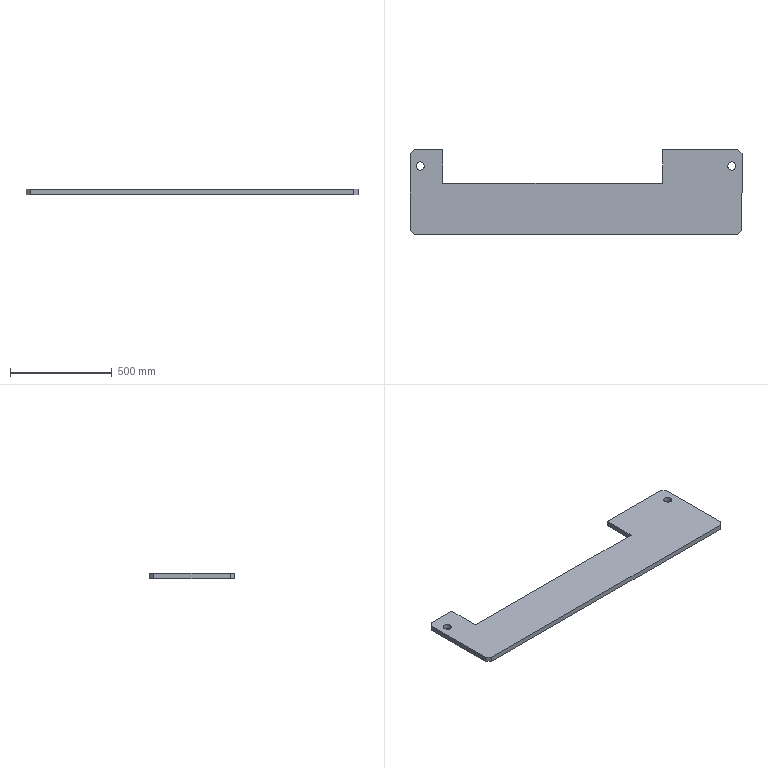Part | SolidWorks | features Chamfer 1, Extrusion 1, ICE 1 | 1 solid | 18 faces | box 1630 x 415 x 25 mm | volume 12373418 mm3 | plane 14 | cylinder 4 | commonest cylinder face diameters 40 x4
STEP:
#1=CARTESIAN_POINT('',(745.,127.5,0.));
#2=VERTEX_POINT('',#1);
#3=CARTESIAN_POINT('',(785.,127.5,0.));
#4=VERTEX_POINT('',#3);
#5=CARTESIAN_POINT('',(765.,127.5,0.));
#6=DIRECTION('',(0.,0.,1.));
#7=DIRECTION('',(1.,0.,0.));
#8=AXIS2_PLACEMENT_3D('',#5,#6,#7);
#9=CIRCLE('',#8,20.);
#10=EDGE_CURVE('',#2,#4,#9,.T.);
#11=ORIENTED_EDGE('',*,*,#10,.F.);
#12=CARTESIAN_POINT('',(745.,127.5,25.));
#13=VERTEX_POINT('',#12);
#14=CARTESIAN_POINT('',(745.,127.5,0.));
#15=DIRECTION('',(0.,0.,1.));
#16=VECTOR('',#15,1000.);
#17=LINE('',#14,#16);
#18=EDGE_CURVE('',#2,#13,#17,.T.);
#19=ORIENTED_EDGE('',*,*,#18,.T.);
#20=CARTESIAN_POINT('',(785.,127.5,25.));
#21=VERTEX_POINT('',#20);
#22=CARTESIAN_POINT('',(765.,127.5,25.));
#23=DIRECTION('',(0.,0.,-1.));
#24=DIRECTION('',(-1.,0.,0.));
#25=AXIS2_PLACEMENT_3D('',#22,#23,#24);
#26=CIRCLE('',#25,20.);
#27=EDGE_CURVE('',#21,#13,#26,.T.);
#28=ORIENTED_EDGE('',*,*,#27,.F.);
#29=CARTESIAN_POINT('',(785.,127.5,0.));
#30=DIRECTION('',(0.,0.,1.));
#31=VECTOR('',#30,1000.);
#32=LINE('',#29,#31);
#33=EDGE_CURVE('',#4,#21,#32,.T.);
#34=ORIENTED_EDGE('',*,*,#33,.F.);
#35=EDGE_LOOP('',(#11,#19,#28,#34));
#36=FACE_OUTER_BOUND('',#35,.T.);
#37=CARTESIAN_POINT('',(765.,127.5,0.));
#38=DIRECTION('',(0.,0.,1.));
#39=DIRECTION('',(1.,0.,0.));
#40=AXIS2_PLACEMENT_3D('',#37,#38,#39);
#41=CYLINDRICAL_SURFACE('',#40,20.);
#42=ADVANCED_FACE('',(#36),#41,.F.);
#43=CARTESIAN_POINT('',(-785.,127.5,0.));
#44=VERTEX_POINT('',#43);
#45=CARTESIAN_POINT('',(-745.,127.5,0.));
#46=VERTEX_POINT('',#45);
#47=CARTESIAN_POINT('',(-765.,127.5,0.));
#48=DIRECTION('',(0.,0.,1.));
#49=DIRECTION('',(1.,0.,0.));
#50=AXIS2_PLACEMENT_3D('',#47,#48,#49);
#51=CIRCLE('',#50,20.);
#52=EDGE_CURVE('',#44,#46,#51,.T.);
#53=ORIENTED_EDGE('',*,*,#52,.F.);
#54=CARTESIAN_POINT('',(-785.,127.5,25.));
#55=VERTEX_POINT('',#54);
#56=CARTESIAN_POINT('',(-785.,127.5,0.));
#57=DIRECTION('',(0.,0.,1.));
#58=VECTOR('',#57,1000.);
#59=LINE('',#56,#58);
#60=EDGE_CURVE('',#44,#55,#59,.T.);
#61=ORIENTED_EDGE('',*,*,#60,.T.);
#62=CARTESIAN_POINT('',(-745.,127.5,25.));
#63=VERTEX_POINT('',#62);
#64=CARTESIAN_POINT('',(-765.,127.5,25.));
#65=DIRECTION('',(0.,0.,-1.));
#66=DIRECTION('',(-1.,0.,0.));
#67=AXIS2_PLACEMENT_3D('',#64,#65,#66);
#68=CIRCLE('',#67,20.);
#69=EDGE_CURVE('',#63,#55,#68,.T.);
#70=ORIENTED_EDGE('',*,*,#69,.F.);
#71=CARTESIAN_POINT('',(-745.,127.5,0.));
#72=DIRECTION('',(0.,0.,1.));
#73=VECTOR('',#72,1000.);
#74=LINE('',#71,#73);
#75=EDGE_CURVE('',#46,#63,#74,.T.);
#76=ORIENTED_EDGE('',*,*,#75,.F.);
#77=EDGE_LOOP('',(#53,#61,#70,#76));
#78=FACE_OUTER_BOUND('',#77,.T.);
#79=CARTESIAN_POINT('',(-765.,127.5,0.));
#80=DIRECTION('',(0.,0.,1.));
#81=DIRECTION('',(1.,0.,0.));
#82=AXIS2_PLACEMENT_3D('',#79,#80,#81);
#83=CYLINDRICAL_SURFACE('',#82,20.);
#84=ADVANCED_FACE('',(#78),#83,.F.);
#85=CARTESIAN_POINT('',(-655.,207.5,25.));
#86=VERTEX_POINT('',#85);
#87=CARTESIAN_POINT('',(-795.,207.5,25.));
#88=VERTEX_POINT('',#87);
#89=CARTESIAN_POINT('',(815.,207.5,25.));
#90=DIRECTION('',(-1.,0.,0.));
#91=VECTOR('',#90,1000.);
#92=LINE('',#89,#91);
#93=EDGE_CURVE('',#86,#88,#92,.T.);
#94=ORIENTED_EDGE('',*,*,#93,.F.);
#95=CARTESIAN_POINT('',(-655.,207.5,0.));
#96=VERTEX_POINT('',#95);
#97=CARTESIAN_POINT('',(-655.,207.5,25.));
#98=DIRECTION('',(0.,0.,-1.));
#99=VECTOR('',#98,1000.);
#100=LINE('',#97,#99);
#101=EDGE_CURVE('',#86,#96,#100,.T.);
#102=ORIENTED_EDGE('',*,*,#101,.T.);
#103=CARTESIAN_POINT('',(-795.,207.5,0.));
#104=VERTEX_POINT('',#103);
#105=CARTESIAN_POINT('',(815.,207.5,0.));
#106=DIRECTION('',(-1.,0.,0.));
#107=VECTOR('',#106,1000.);
#108=LINE('',#105,#107);
#109=EDGE_CURVE('',#96,#104,#108,.T.);
#110=ORIENTED_EDGE('',*,*,#109,.T.);
#111=CARTESIAN_POINT('',(-795.,207.5,25.));
#112=DIRECTION('',(0.,0.,1.));
#113=VECTOR('',#112,1000.);
#114=LINE('',#111,#113);
#115=EDGE_CURVE('',#104,#88,#114,.T.);
#116=ORIENTED_EDGE('',*,*,#115,.T.);
#117=EDGE_LOOP('',(#94,#102,#110,#116));
#118=FACE_OUTER_BOUND('',#117,.T.);
#119=CARTESIAN_POINT('',(815.,207.5,25.));
#120=DIRECTION('',(0.,-1.,0.));
#121=DIRECTION('',(1.,0.,0.));
#122=AXIS2_PLACEMENT_3D('',#119,#120,#121);
#123=PLANE('',#122);
#124=ADVANCED_FACE('',(#118),#123,.F.);
#125=CARTESIAN_POINT('',(-815.,187.5,0.));
#126=VERTEX_POINT('',#125);
#127=CARTESIAN_POINT('',(-815.,-187.5,0.));
#128=VERTEX_POINT('',#127);
#129=CARTESIAN_POINT('',(-815.,207.5,0.));
#130=DIRECTION('',(0.,-1.,0.));
#131=VECTOR('',#130,1000.);
#132=LINE('',#129,#131);
#133=EDGE_CURVE('',#126,#128,#132,.T.);
#134=ORIENTED_EDGE('',*,*,#133,.T.);
#135=CARTESIAN_POINT('',(-815.,-187.5,25.));
#136=VERTEX_POINT('',#135);
#137=CARTESIAN_POINT('',(-815.,-187.5,25.));
#138=DIRECTION('',(0.,0.,1.));
#139=VECTOR('',#138,1000.);
#140=LINE('',#137,#139);
#141=EDGE_CURVE('',#128,#136,#140,.T.);
#142=ORIENTED_EDGE('',*,*,#141,.T.);
#143=CARTESIAN_POINT('',(-815.,187.5,25.));
#144=VERTEX_POINT('',#143);
#145=CARTESIAN_POINT('',(-815.,207.5,25.));
#146=DIRECTION('',(0.,-1.,0.));
#147=VECTOR('',#146,1000.);
#148=LINE('',#145,#147);
#149=EDGE_CURVE('',#144,#136,#148,.T.);
#150=ORIENTED_EDGE('',*,*,#149,.F.);
#151=CARTESIAN_POINT('',(-815.,187.5,25.));
#152=DIRECTION('',(0.,0.,-1.));
#153=VECTOR('',#152,1000.);
#154=LINE('',#151,#153);
#155=EDGE_CURVE('',#144,#126,#154,.T.);
#156=ORIENTED_EDGE('',*,*,#155,.T.);
#157=EDGE_LOOP('',(#134,#142,#150,#156));
#158=FACE_OUTER_BOUND('',#157,.T.);
#159=CARTESIAN_POINT('',(-815.,207.5,25.));
#160=DIRECTION('',(1.,0.,0.));
#161=DIRECTION('',(0.,1.,0.));
#162=AXIS2_PLACEMENT_3D('',#159,#160,#161);
#163=PLANE('',#162);
#164=ADVANCED_FACE('',(#158),#163,.F.);
#165=CARTESIAN_POINT('',(-795.,-207.5,25.));
#166=VERTEX_POINT('',#165);
#167=CARTESIAN_POINT('',(795.,-207.5,25.));
#168=VERTEX_POINT('',#167);
#169=CARTESIAN_POINT('',(815.,-207.5,25.));
#170=DIRECTION('',(1.,0.,0.));
#171=VECTOR('',#170,1000.);
#172=LINE('',#169,#171);
#173=EDGE_CURVE('',#166,#168,#172,.T.);
#174=ORIENTED_EDGE('',*,*,#173,.F.);
#175=CARTESIAN_POINT('',(-795.,-207.5,0.));
#176=VERTEX_POINT('',#175);
#177=CARTESIAN_POINT('',(-795.,-207.5,25.));
#178=DIRECTION('',(0.,0.,-1.));
#179=VECTOR('',#178,1000.);
#180=LINE('',#177,#179);
#181=EDGE_CURVE('',#166,#176,#180,.T.);
#182=ORIENTED_EDGE('',*,*,#181,.T.);
#183=CARTESIAN_POINT('',(795.,-207.5,0.));
#184=VERTEX_POINT('',#183);
#185=CARTESIAN_POINT('',(815.,-207.5,0.));
#186=DIRECTION('',(1.,0.,0.));
#187=VECTOR('',#186,1000.);
#188=LINE('',#185,#187);
#189=EDGE_CURVE('',#176,#184,#188,.T.);
#190=ORIENTED_EDGE('',*,*,#189,.T.);
#191=CARTESIAN_POINT('',(795.,-207.5,25.));
#192=DIRECTION('',(0.,0.,1.));
#193=VECTOR('',#192,1000.);
#194=LINE('',#191,#193);
#195=EDGE_CURVE('',#184,#168,#194,.T.);
#196=ORIENTED_EDGE('',*,*,#195,.T.);
#197=EDGE_LOOP('',(#174,#182,#190,#196));
#198=FACE_OUTER_BOUND('',#197,.T.);
#199=CARTESIAN_POINT('',(815.,-207.5,25.));
#200=DIRECTION('',(0.,1.,0.));
#201=DIRECTION('',(-1.,0.,0.));
#202=AXIS2_PLACEMENT_3D('',#199,#200,#201);
#203=PLANE('',#202);
#204=ADVANCED_FACE('',(#198),#203,.F.);
#205=CARTESIAN_POINT('',(815.,-187.5,25.));
#206=VERTEX_POINT('',#205);
#207=CARTESIAN_POINT('',(815.,187.5,25.));
#208=VERTEX_POINT('',#207);
#209=CARTESIAN_POINT('',(815.,207.5,25.));
#210=DIRECTION('',(0.,1.,0.));
#211=VECTOR('',#210,1000.);
#212=LINE('',#209,#211);
#213=EDGE_CURVE('',#206,#208,#212,.T.);
#214=ORIENTED_EDGE('',*,*,#213,.F.);
#215=CARTESIAN_POINT('',(815.,-187.5,0.));
#216=VERTEX_POINT('',#215);
#217=CARTESIAN_POINT('',(815.,-187.5,25.));
#218=DIRECTION('',(0.,0.,-1.));
#219=VECTOR('',#218,1000.);
#220=LINE('',#217,#219);
#221=EDGE_CURVE('',#206,#216,#220,.T.);
#222=ORIENTED_EDGE('',*,*,#221,.T.);
#223=CARTESIAN_POINT('',(815.,187.5,0.));
#224=VERTEX_POINT('',#223);
#225=CARTESIAN_POINT('',(815.,207.5,0.));
#226=DIRECTION('',(0.,1.,0.));
#227=VECTOR('',#226,1000.);
#228=LINE('',#225,#227);
#229=EDGE_CURVE('',#216,#224,#228,.T.);
#230=ORIENTED_EDGE('',*,*,#229,.T.);
#231=CARTESIAN_POINT('',(815.,187.5,25.));
#232=DIRECTION('',(0.,0.,1.));
#233=VECTOR('',#232,1000.);
#234=LINE('',#231,#233);
#235=EDGE_CURVE('',#224,#208,#234,.T.);
#236=ORIENTED_EDGE('',*,*,#235,.T.);
#237=EDGE_LOOP('',(#214,#222,#230,#236));
#238=FACE_OUTER_BOUND('',#237,.T.);
#239=CARTESIAN_POINT('',(815.,207.5,25.));
#240=DIRECTION('',(-1.,0.,0.));
#241=DIRECTION('',(0.,-1.,0.));
#242=AXIS2_PLACEMENT_3D('',#239,#240,#241);
#243=PLANE('',#242);
#244=ADVANCED_FACE('',(#238),#243,.F.);
#245=CARTESIAN_POINT('',(795.,207.5,0.));
#246=VERTEX_POINT('',#245);
#247=CARTESIAN_POINT('',(425.,207.5,0.));
#248=VERTEX_POINT('',#247);
#249=CARTESIAN_POINT('',(815.,207.5,0.));
#250=DIRECTION('',(-1.,0.,0.));
#251=VECTOR('',#250,1000.);
#252=LINE('',#249,#251);
#253=EDGE_CURVE('',#246,#248,#252,.T.);
#254=ORIENTED_EDGE('',*,*,#253,.T.);
#255=CARTESIAN_POINT('',(425.,207.5,25.));
#256=VERTEX_POINT('',#255);
#257=CARTESIAN_POINT('',(425.,207.5,25.));
#258=DIRECTION('',(0.,0.,1.));
#259=VECTOR('',#258,1000.);
#260=LINE('',#257,#259);
#261=EDGE_CURVE('',#248,#256,#260,.T.);
#262=ORIENTED_EDGE('',*,*,#261,.T.);
#263=CARTESIAN_POINT('',(795.,207.5,25.));
#264=VERTEX_POINT('',#263);
#265=CARTESIAN_POINT('',(815.,207.5,25.));
#266=DIRECTION('',(-1.,0.,0.));
#267=VECTOR('',#266,1000.);
#268=LINE('',#265,#267);
#269=EDGE_CURVE('',#264,#256,#268,.T.);
#270=ORIENTED_EDGE('',*,*,#269,.F.);
#271=CARTESIAN_POINT('',(795.,207.5,25.));
#272=DIRECTION('',(0.,0.,-1.));
#273=VECTOR('',#272,1000.);
#274=LINE('',#271,#273);
#275=EDGE_CURVE('',#264,#246,#274,.T.);
#276=ORIENTED_EDGE('',*,*,#275,.T.);
#277=EDGE_LOOP('',(#254,#262,#270,#276));
#278=FACE_OUTER_BOUND('',#277,.T.);
#279=CARTESIAN_POINT('',(815.,207.5,25.));
#280=DIRECTION('',(0.,-1.,0.));
#281=DIRECTION('',(1.,0.,0.));
#282=AXIS2_PLACEMENT_3D('',#279,#280,#281);
#283=PLANE('',#282);
#284=ADVANCED_FACE('',(#278),#283,.F.);
#285=ORIENTED_EDGE('',*,*,#27,.T.);
#286=CARTESIAN_POINT('',(765.,127.5,25.));
#287=DIRECTION('',(0.,0.,-1.));
#288=DIRECTION('',(-1.,0.,0.));
#289=AXIS2_PLACEMENT_3D('',#286,#287,#288);
#290=CIRCLE('',#289,20.);
#291=EDGE_CURVE('',#13,#21,#290,.T.);
#292=ORIENTED_EDGE('',*,*,#291,.T.);
#293=EDGE_LOOP('',(#285,#292));
#294=FACE_BOUND('',#293,.T.);
#295=ORIENTED_EDGE('',*,*,#69,.T.);
#296=CARTESIAN_POINT('',(-765.,127.5,25.));
#297=DIRECTION('',(0.,0.,-1.));
#298=DIRECTION('',(-1.,0.,0.));
#299=AXIS2_PLACEMENT_3D('',#296,#297,#298);
#300=CIRCLE('',#299,20.);
#301=EDGE_CURVE('',#55,#63,#300,.T.);
#302=ORIENTED_EDGE('',*,*,#301,.T.);
#303=EDGE_LOOP('',(#295,#302));
#304=FACE_BOUND('',#303,.T.);
#305=CARTESIAN_POINT('',(425.,42.5,25.));
#306=VERTEX_POINT('',#305);
#307=CARTESIAN_POINT('',(-655.,42.5,25.));
#308=VERTEX_POINT('',#307);
#309=CARTESIAN_POINT('',(0.,42.5,25.));
#310=DIRECTION('',(-1.,0.,0.));
#311=VECTOR('',#310,1000.);
#312=LINE('',#309,#311);
#313=EDGE_CURVE('',#306,#308,#312,.T.);
#314=ORIENTED_EDGE('',*,*,#313,.T.);
#315=CARTESIAN_POINT('',(-655.,0.,25.));
#316=DIRECTION('',(0.,1.,0.));
#317=VECTOR('',#316,1000.);
#318=LINE('',#315,#317);
#319=EDGE_CURVE('',#308,#86,#318,.T.);
#320=ORIENTED_EDGE('',*,*,#319,.T.);
#321=ORIENTED_EDGE('',*,*,#93,.T.);
#322=CARTESIAN_POINT('',(-815.,187.5,25.));
#323=DIRECTION('',(-0.7071,-0.7071,0.));
#324=VECTOR('',#323,1000.);
#325=LINE('',#322,#324);
#326=EDGE_CURVE('',#88,#144,#325,.T.);
#327=ORIENTED_EDGE('',*,*,#326,.T.);
#328=ORIENTED_EDGE('',*,*,#149,.T.);
#329=CARTESIAN_POINT('',(-795.,-207.5,25.));
#330=DIRECTION('',(0.7071,-0.7071,0.));
#331=VECTOR('',#330,1000.);
#332=LINE('',#329,#331);
#333=EDGE_CURVE('',#136,#166,#332,.T.);
#334=ORIENTED_EDGE('',*,*,#333,.T.);
#335=ORIENTED_EDGE('',*,*,#173,.T.);
#336=CARTESIAN_POINT('',(815.,-187.5,25.));
#337=DIRECTION('',(0.7071,0.7071,0.));
#338=VECTOR('',#337,1000.);
#339=LINE('',#336,#338);
#340=EDGE_CURVE('',#168,#206,#339,.T.);
#341=ORIENTED_EDGE('',*,*,#340,.T.);
#342=ORIENTED_EDGE('',*,*,#213,.T.);
#343=CARTESIAN_POINT('',(795.,207.5,25.));
#344=DIRECTION('',(-0.7071,0.7071,0.));
#345=VECTOR('',#344,1000.);
#346=LINE('',#343,#345);
#347=EDGE_CURVE('',#208,#264,#346,.T.);
#348=ORIENTED_EDGE('',*,*,#347,.T.);
#349=ORIENTED_EDGE('',*,*,#269,.T.);
#350=CARTESIAN_POINT('',(425.,0.,25.));
#351=DIRECTION('',(0.,-1.,0.));
#352=VECTOR('',#351,1000.);
#353=LINE('',#350,#352);
#354=EDGE_CURVE('',#256,#306,#353,.T.);
#355=ORIENTED_EDGE('',*,*,#354,.T.);
#356=EDGE_LOOP('',(#314,#320,#321,#327,#328,#334,#335,#341,#342,#348,#349,#355));
#357=FACE_OUTER_BOUND('',#356,.T.);
#358=CARTESIAN_POINT('',(0.,0.,25.));
#359=DIRECTION('',(0.,0.,-1.));
#360=DIRECTION('',(-1.,0.,0.));
#361=AXIS2_PLACEMENT_3D('',#358,#359,#360);
#362=PLANE('',#361);
#363=ADVANCED_FACE('',(#294,#304,#357),#362,.F.);
#364=CARTESIAN_POINT('',(765.,127.5,0.));
#365=DIRECTION('',(0.,0.,1.));
#366=DIRECTION('',(1.,0.,0.));
#367=AXIS2_PLACEMENT_3D('',#364,#365,#366);
#368=CIRCLE('',#367,20.);
#369=EDGE_CURVE('',#4,#2,#368,.T.);
#370=ORIENTED_EDGE('',*,*,#369,.T.);
#371=ORIENTED_EDGE('',*,*,#10,.T.);
#372=EDGE_LOOP('',(#370,#371));
#373=FACE_BOUND('',#372,.T.);
#374=CARTESIAN_POINT('',(-765.,127.5,0.));
#375=DIRECTION('',(0.,0.,1.));
#376=DIRECTION('',(1.,0.,0.));
#377=AXIS2_PLACEMENT_3D('',#374,#375,#376);
#378=CIRCLE('',#377,20.);
#379=EDGE_CURVE('',#46,#44,#378,.T.);
#380=ORIENTED_EDGE('',*,*,#379,.T.);
#381=ORIENTED_EDGE('',*,*,#52,.T.);
#382=EDGE_LOOP('',(#380,#381));
#383=FACE_BOUND('',#382,.T.);
#384=CARTESIAN_POINT('',(-655.,42.5,0.));
#385=VERTEX_POINT('',#384);
#386=CARTESIAN_POINT('',(-655.,0.,0.));
#387=DIRECTION('',(0.,1.,0.));
#388=VECTOR('',#387,1000.);
#389=LINE('',#386,#388);
#390=EDGE_CURVE('',#385,#96,#389,.T.);
#391=ORIENTED_EDGE('',*,*,#390,.F.);
#392=CARTESIAN_POINT('',(425.,42.5,0.));
#393=VERTEX_POINT('',#392);
#394=CARTESIAN_POINT('',(-655.,42.5,0.));
#395=DIRECTION('',(1.,0.,0.));
#396=VECTOR('',#395,1000.);
#397=LINE('',#394,#396);
#398=EDGE_CURVE('',#385,#393,#397,.T.);
#399=ORIENTED_EDGE('',*,*,#398,.T.);
#400=CARTESIAN_POINT('',(425.,42.5,0.));
#401=DIRECTION('',(0.,1.,0.));
#402=VECTOR('',#401,1000.);
#403=LINE('',#400,#402);
#404=EDGE_CURVE('',#393,#248,#403,.T.);
#405=ORIENTED_EDGE('',*,*,#404,.T.);
#406=ORIENTED_EDGE('',*,*,#253,.F.);
#407=CARTESIAN_POINT('',(501.25,501.25,0.));
#408=DIRECTION('',(0.7071,-0.7071,0.));
#409=VECTOR('',#408,1000.);
#410=LINE('',#407,#409);
#411=EDGE_CURVE('',#246,#224,#410,.T.);
#412=ORIENTED_EDGE('',*,*,#411,.T.);
#413=ORIENTED_EDGE('',*,*,#229,.F.);
#414=CARTESIAN_POINT('',(501.25,-501.25,0.));
#415=DIRECTION('',(-0.7071,-0.7071,0.));
#416=VECTOR('',#415,1000.);
#417=LINE('',#414,#416);
#418=EDGE_CURVE('',#216,#184,#417,.T.);
#419=ORIENTED_EDGE('',*,*,#418,.T.);
#420=ORIENTED_EDGE('',*,*,#189,.F.);
#421=CARTESIAN_POINT('',(-501.25,-501.25,0.));
#422=DIRECTION('',(-0.7071,0.7071,0.));
#423=VECTOR('',#422,1000.);
#424=LINE('',#421,#423);
#425=EDGE_CURVE('',#176,#128,#424,.T.);
#426=ORIENTED_EDGE('',*,*,#425,.T.);
#427=ORIENTED_EDGE('',*,*,#133,.F.);
#428=CARTESIAN_POINT('',(-501.25,501.25,0.));
#429=DIRECTION('',(0.7071,0.7071,0.));
#430=VECTOR('',#429,1000.);
#431=LINE('',#428,#430);
#432=EDGE_CURVE('',#126,#104,#431,.T.);
#433=ORIENTED_EDGE('',*,*,#432,.T.);
#434=ORIENTED_EDGE('',*,*,#109,.F.);
#435=EDGE_LOOP('',(#391,#399,#405,#406,#412,#413,#419,#420,#426,#427,#433,#434));
#436=FACE_OUTER_BOUND('',#435,.T.);
#437=CARTESIAN_POINT('',(0.,0.,0.));
#438=DIRECTION('',(0.,0.,-1.));
#439=DIRECTION('',(-1.,0.,0.));
#440=AXIS2_PLACEMENT_3D('',#437,#438,#439);
#441=PLANE('',#440);
#442=ADVANCED_FACE('',(#373,#383,#436),#441,.T.);
#443=ORIENTED_EDGE('',*,*,#333,.F.);
#444=ORIENTED_EDGE('',*,*,#141,.F.);
#445=ORIENTED_EDGE('',*,*,#425,.F.);
#446=ORIENTED_EDGE('',*,*,#181,.F.);
#447=EDGE_LOOP('',(#443,#444,#445,#446));
#448=FACE_OUTER_BOUND('',#447,.T.);
#449=CARTESIAN_POINT('',(-795.,-207.5,25.));
#450=DIRECTION('',(0.7071,0.7071,0.));
#451=DIRECTION('',(0.,0.,-1.));
#452=AXIS2_PLACEMENT_3D('',#449,#450,#451);
#453=PLANE('',#452);
#454=ADVANCED_FACE('',(#448),#453,.F.);
#455=ORIENTED_EDGE('',*,*,#340,.F.);
#456=ORIENTED_EDGE('',*,*,#195,.F.);
#457=ORIENTED_EDGE('',*,*,#418,.F.);
#458=ORIENTED_EDGE('',*,*,#221,.F.);
#459=EDGE_LOOP('',(#455,#456,#457,#458));
#460=FACE_OUTER_BOUND('',#459,.T.);
#461=CARTESIAN_POINT('',(815.,-187.5,25.));
#462=DIRECTION('',(-0.7071,0.7071,0.));
#463=DIRECTION('',(0.,0.,-1.));
#464=AXIS2_PLACEMENT_3D('',#461,#462,#463);
#465=PLANE('',#464);
#466=ADVANCED_FACE('',(#460),#465,.F.);
#467=ORIENTED_EDGE('',*,*,#347,.F.);
#468=ORIENTED_EDGE('',*,*,#235,.F.);
#469=ORIENTED_EDGE('',*,*,#411,.F.);
#470=ORIENTED_EDGE('',*,*,#275,.F.);
#471=EDGE_LOOP('',(#467,#468,#469,#470));
#472=FACE_OUTER_BOUND('',#471,.T.);
#473=CARTESIAN_POINT('',(795.,207.5,25.));
#474=DIRECTION('',(-0.7071,-0.7071,0.));
#475=DIRECTION('',(0.,0.,-1.));
#476=AXIS2_PLACEMENT_3D('',#473,#474,#475);
#477=PLANE('',#476);
#478=ADVANCED_FACE('',(#472),#477,.F.);
#479=ORIENTED_EDGE('',*,*,#326,.F.);
#480=ORIENTED_EDGE('',*,*,#115,.F.);
#481=ORIENTED_EDGE('',*,*,#432,.F.);
#482=ORIENTED_EDGE('',*,*,#155,.F.);
#483=EDGE_LOOP('',(#479,#480,#481,#482));
#484=FACE_OUTER_BOUND('',#483,.T.);
#485=CARTESIAN_POINT('',(-815.,187.5,25.));
#486=DIRECTION('',(0.7071,-0.7071,0.));
#487=DIRECTION('',(0.,0.,-1.));
#488=AXIS2_PLACEMENT_3D('',#485,#486,#487);
#489=PLANE('',#488);
#490=ADVANCED_FACE('',(#484),#489,.F.);
#491=ORIENTED_EDGE('',*,*,#319,.F.);
#492=CARTESIAN_POINT('',(-655.,42.5,0.));
#493=DIRECTION('',(0.,0.,1.));
#494=VECTOR('',#493,1000.);
#495=LINE('',#492,#494);
#496=EDGE_CURVE('',#385,#308,#495,.T.);
#497=ORIENTED_EDGE('',*,*,#496,.F.);
#498=ORIENTED_EDGE('',*,*,#390,.T.);
#499=ORIENTED_EDGE('',*,*,#101,.F.);
#500=EDGE_LOOP('',(#491,#497,#498,#499));
#501=FACE_OUTER_BOUND('',#500,.T.);
#502=CARTESIAN_POINT('',(-655.,42.5,0.));
#503=DIRECTION('',(-1.,0.,0.));
#504=DIRECTION('',(0.,-1.,0.));
#505=AXIS2_PLACEMENT_3D('',#502,#503,#504);
#506=PLANE('',#505);
#507=ADVANCED_FACE('',(#501),#506,.F.);
#508=ORIENTED_EDGE('',*,*,#404,.F.);
#509=CARTESIAN_POINT('',(425.,42.5,0.));
#510=DIRECTION('',(0.,0.,1.));
#511=VECTOR('',#510,1000.);
#512=LINE('',#509,#511);
#513=EDGE_CURVE('',#393,#306,#512,.T.);
#514=ORIENTED_EDGE('',*,*,#513,.T.);
#515=ORIENTED_EDGE('',*,*,#354,.F.);
#516=ORIENTED_EDGE('',*,*,#261,.F.);
#517=EDGE_LOOP('',(#508,#514,#515,#516));
#518=FACE_OUTER_BOUND('',#517,.T.);
#519=CARTESIAN_POINT('',(425.,42.5,0.));
#520=DIRECTION('',(1.,0.,0.));
#521=DIRECTION('',(0.,1.,0.));
#522=AXIS2_PLACEMENT_3D('',#519,#520,#521);
#523=PLANE('',#522);
#524=ADVANCED_FACE('',(#518),#523,.F.);
#525=ORIENTED_EDGE('',*,*,#513,.F.);
#526=ORIENTED_EDGE('',*,*,#398,.F.);
#527=ORIENTED_EDGE('',*,*,#496,.T.);
#528=ORIENTED_EDGE('',*,*,#313,.F.);
#529=EDGE_LOOP('',(#525,#526,#527,#528));
#530=FACE_OUTER_BOUND('',#529,.T.);
#531=CARTESIAN_POINT('',(-655.,42.5,0.));
#532=DIRECTION('',(0.,-1.,0.));
#533=DIRECTION('',(0.,0.,-1.));
#534=AXIS2_PLACEMENT_3D('',#531,#532,#533);
#535=PLANE('',#534);
#536=ADVANCED_FACE('',(#530),#535,.F.);
#537=ORIENTED_EDGE('',*,*,#60,.F.);
#538=ORIENTED_EDGE('',*,*,#379,.F.);
#539=ORIENTED_EDGE('',*,*,#75,.T.);
#540=ORIENTED_EDGE('',*,*,#301,.F.);
#541=EDGE_LOOP('',(#537,#538,#539,#540));
#542=FACE_OUTER_BOUND('',#541,.T.);
#543=CARTESIAN_POINT('',(-765.,127.5,0.));
#544=DIRECTION('',(0.,0.,1.));
#545=DIRECTION('',(1.,0.,0.));
#546=AXIS2_PLACEMENT_3D('',#543,#544,#545);
#547=CYLINDRICAL_SURFACE('',#546,20.);
#548=ADVANCED_FACE('',(#542),#547,.F.);
#549=ORIENTED_EDGE('',*,*,#18,.F.);
#550=ORIENTED_EDGE('',*,*,#369,.F.);
#551=ORIENTED_EDGE('',*,*,#33,.T.);
#552=ORIENTED_EDGE('',*,*,#291,.F.);
#553=EDGE_LOOP('',(#549,#550,#551,#552));
#554=FACE_OUTER_BOUND('',#553,.T.);
#555=CARTESIAN_POINT('',(765.,127.5,0.));
#556=DIRECTION('',(0.,0.,1.));
#557=DIRECTION('',(1.,0.,0.));
#558=AXIS2_PLACEMENT_3D('',#555,#556,#557);
#559=CYLINDRICAL_SURFACE('',#558,20.);
#560=ADVANCED_FACE('',(#554),#559,.F.);
#561=CLOSED_SHELL('',(#42,#84,#124,#164,#204,#244,#284,#363,#442,#454,#466,#478,#490,#507,#524,#536,#548,#560));
#562=MANIFOLD_SOLID_BREP('',#561);
#563=CARTESIAN_POINT('',(0.,0.,0.));
#564=DIRECTION('',(0.,0.,1.));
#565=DIRECTION('',(1.,0.,0.));
#566=AXIS2_PLACEMENT_3D('',#563,#564,#565);
#567=(LENGTH_UNIT()NAMED_UNIT(*)SI_UNIT(.MILLI.,.METRE.));
#568=UNCERTAINTY_MEASURE_WITH_UNIT(LENGTH_MEASURE(0.00001),#567,'','');
#569=(NAMED_UNIT(*)PLANE_ANGLE_UNIT()SI_UNIT($,.RADIAN.));
#570=(NAMED_UNIT(*)SI_UNIT($,.STERADIAN.)SOLID_ANGLE_UNIT());
#571=(GEOMETRIC_REPRESENTATION_CONTEXT(3)GLOBAL_UNCERTAINTY_ASSIGNED_CONTEXT((#568))GLOBAL_UNIT_ASSIGNED_CONTEXT((#567,#569,#570))REPRESENTATION_CONTEXT('',''));
#572=ADVANCED_BREP_SHAPE_REPRESENTATION('',(#562,#566),#571);